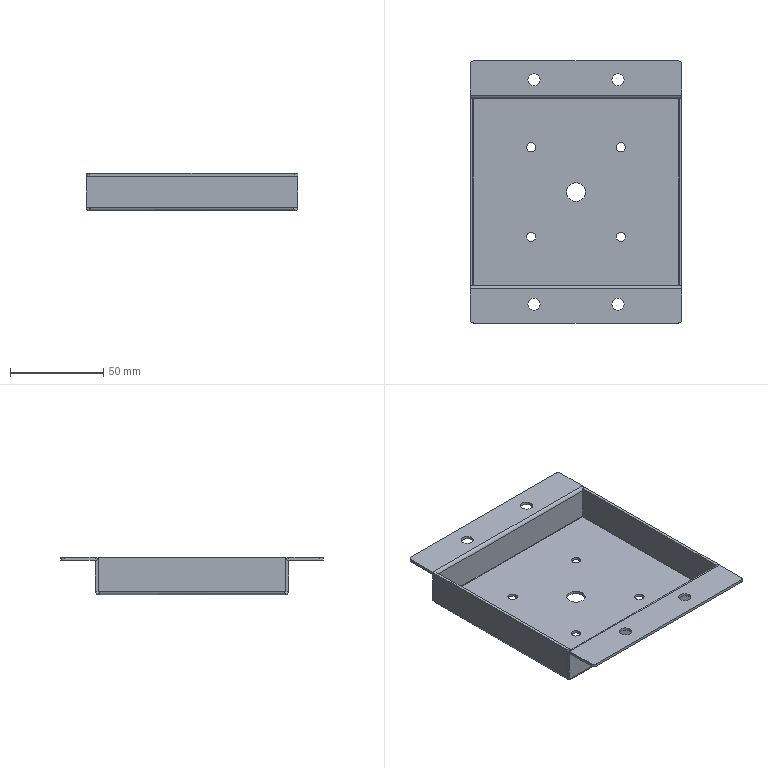Part | STEP file | FBDS-BJ-017 | 1 solid | 84 faces | box 113.4 x 140.4 x 20 mm | volume 34877 mm3 | plane 42 | cylinder 34 | spline 8 | commonest cylinder face diameters 5 x8 6.5 x8 0.4 x6 3.4 x6 4 x4 10 x2